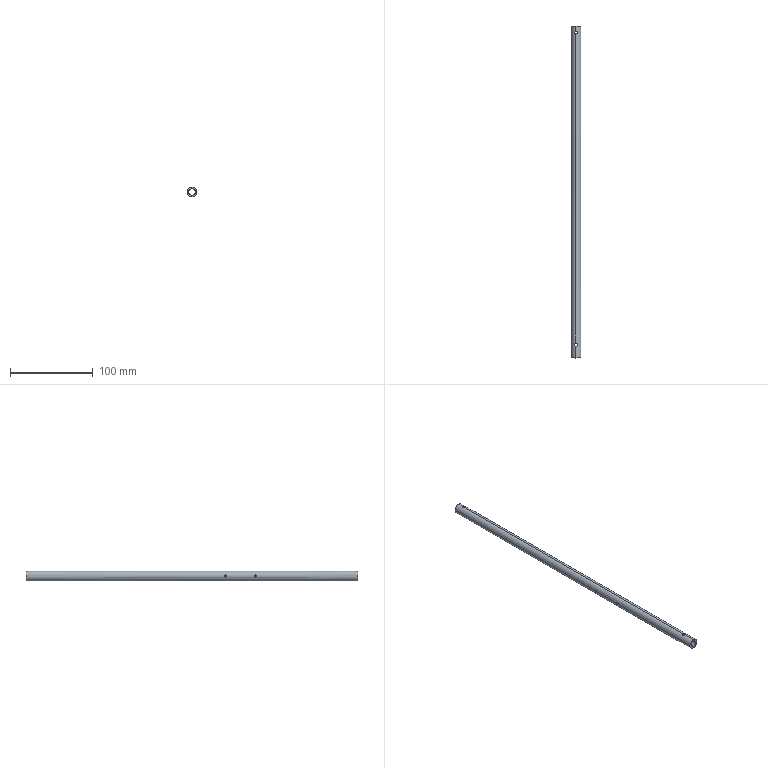Part | SolidWorks | features ICE 2, Extrusion 1 | 1 solid | 22 faces | box 12 x 400 x 12 mm | volume 25005 mm3 | cylinder 20 | plane 2 | commonest cylinder face diameters 2.6 x8 3.1 x4 4.1 x4 8 x2 12 x2